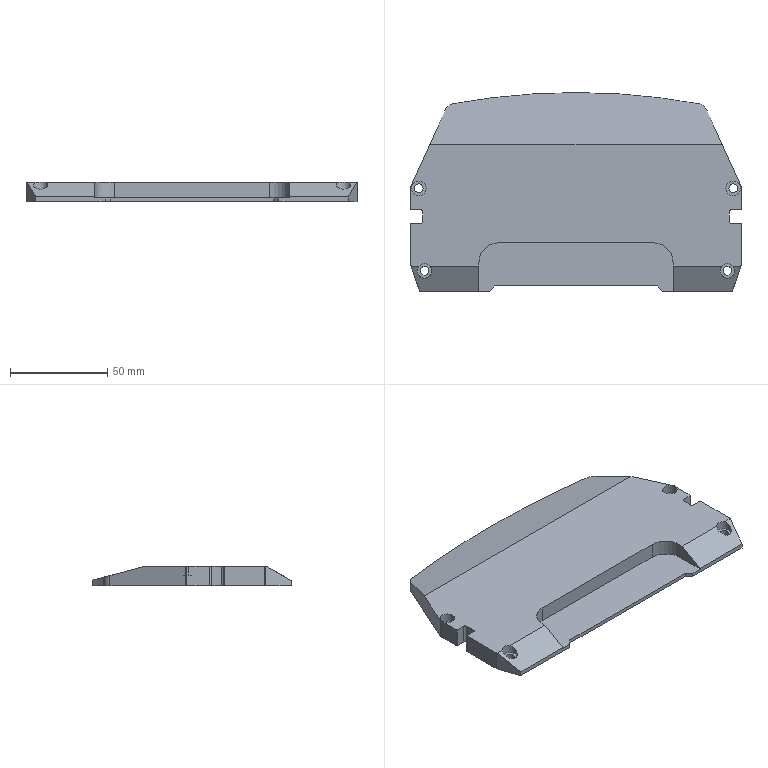Part | STEP file | 复件 FHB175-001^FHB175S-PRW-P40(马达RightUpper折-400W伺服电机) | 1 solid | 65 faces | box 170 x 102.4 x 10 mm | volume 124038 mm3 | cylinder 33 | plane 32 | commonest cylinder face diameters 2 x8 4.5 x8 7.5 x8 0.6 x4 10 x2 20 x2